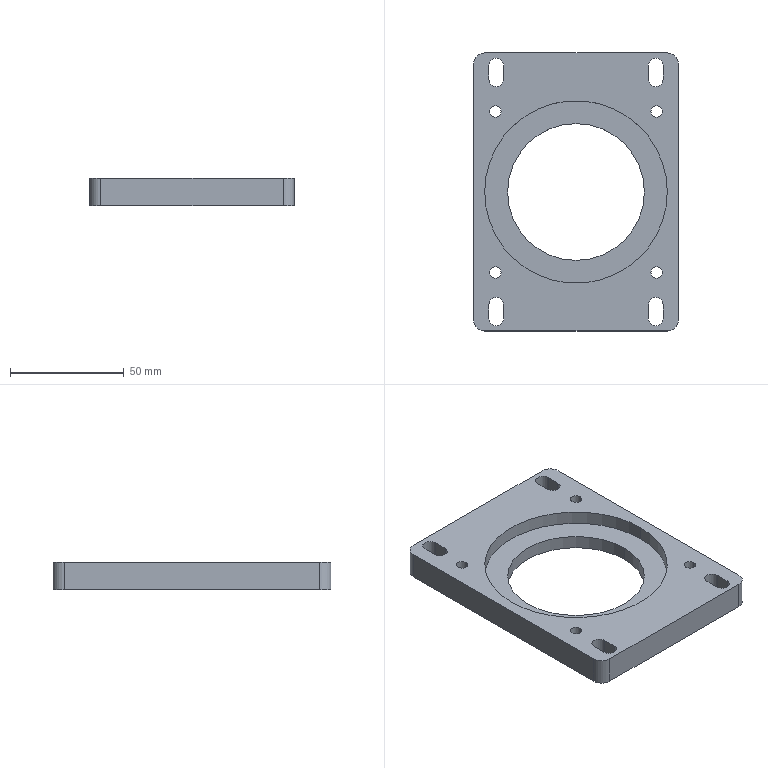Part | SolidWorks | features ICE 3, Extrusion 1, Fillet 1, HoleWzd 1 | 1 solid | 39 faces | box 90 x 122 x 12 mm | volume 79896 mm3 | cylinder 24 | plane 15 | commonest cylinder face diameters 5 x8 6.5 x8 10 x4 60 x2 80.1 x2
STEP:
#1=CARTESIAN_POINT('',(32.855,35.355,0.));
#2=VERTEX_POINT('',#1);
#3=CARTESIAN_POINT('',(37.855,35.355,0.));
#4=VERTEX_POINT('',#3);
#5=CARTESIAN_POINT('',(35.355,35.355,0.));
#6=DIRECTION('',(0.,0.,1.));
#7=DIRECTION('',(1.,0.,0.));
#8=AXIS2_PLACEMENT_3D('',#5,#6,#7);
#9=CIRCLE('',#8,2.5);
#10=EDGE_CURVE('',#2,#4,#9,.T.);
#11=ORIENTED_EDGE('',*,*,#10,.F.);
#12=CARTESIAN_POINT('',(32.855,35.355,12.));
#13=VERTEX_POINT('',#12);
#14=CARTESIAN_POINT('',(32.855,35.355,12.));
#15=DIRECTION('',(0.,0.,1.));
#16=VECTOR('',#15,1000.);
#17=LINE('',#14,#16);
#18=EDGE_CURVE('',#2,#13,#17,.T.);
#19=ORIENTED_EDGE('',*,*,#18,.T.);
#20=CARTESIAN_POINT('',(37.855,35.355,12.));
#21=VERTEX_POINT('',#20);
#22=CARTESIAN_POINT('',(35.355,35.355,12.));
#23=DIRECTION('',(0.,0.,1.));
#24=DIRECTION('',(1.,0.,0.));
#25=AXIS2_PLACEMENT_3D('',#22,#23,#24);
#26=CIRCLE('',#25,2.5);
#27=EDGE_CURVE('',#13,#21,#26,.T.);
#28=ORIENTED_EDGE('',*,*,#27,.T.);
#29=CARTESIAN_POINT('',(37.855,35.355,12.));
#30=DIRECTION('',(0.,0.,1.));
#31=VECTOR('',#30,1000.);
#32=LINE('',#29,#31);
#33=EDGE_CURVE('',#4,#21,#32,.T.);
#34=ORIENTED_EDGE('',*,*,#33,.F.);
#35=EDGE_LOOP('',(#11,#19,#28,#34));
#36=FACE_OUTER_BOUND('',#35,.T.);
#37=CARTESIAN_POINT('',(35.355,35.355,12.));
#38=DIRECTION('',(0.,0.,1.));
#39=DIRECTION('',(1.,0.,0.));
#40=AXIS2_PLACEMENT_3D('',#37,#38,#39);
#41=CYLINDRICAL_SURFACE('',#40,2.5);
#42=ADVANCED_FACE('',(#36),#41,.F.);
#43=CARTESIAN_POINT('',(-37.855,35.355,0.));
#44=VERTEX_POINT('',#43);
#45=CARTESIAN_POINT('',(-32.855,35.355,0.));
#46=VERTEX_POINT('',#45);
#47=CARTESIAN_POINT('',(-35.355,35.355,0.));
#48=DIRECTION('',(0.,0.,1.));
#49=DIRECTION('',(1.,0.,0.));
#50=AXIS2_PLACEMENT_3D('',#47,#48,#49);
#51=CIRCLE('',#50,2.5);
#52=EDGE_CURVE('',#44,#46,#51,.T.);
#53=ORIENTED_EDGE('',*,*,#52,.F.);
#54=CARTESIAN_POINT('',(-37.855,35.355,12.));
#55=VERTEX_POINT('',#54);
#56=CARTESIAN_POINT('',(-37.855,35.355,12.));
#57=DIRECTION('',(0.,0.,1.));
#58=VECTOR('',#57,1000.);
#59=LINE('',#56,#58);
#60=EDGE_CURVE('',#44,#55,#59,.T.);
#61=ORIENTED_EDGE('',*,*,#60,.T.);
#62=CARTESIAN_POINT('',(-32.855,35.355,12.));
#63=VERTEX_POINT('',#62);
#64=CARTESIAN_POINT('',(-35.355,35.355,12.));
#65=DIRECTION('',(0.,0.,1.));
#66=DIRECTION('',(1.,0.,0.));
#67=AXIS2_PLACEMENT_3D('',#64,#65,#66);
#68=CIRCLE('',#67,2.5);
#69=EDGE_CURVE('',#55,#63,#68,.T.);
#70=ORIENTED_EDGE('',*,*,#69,.T.);
#71=CARTESIAN_POINT('',(-32.855,35.355,12.));
#72=DIRECTION('',(0.,0.,1.));
#73=VECTOR('',#72,1000.);
#74=LINE('',#71,#73);
#75=EDGE_CURVE('',#46,#63,#74,.T.);
#76=ORIENTED_EDGE('',*,*,#75,.F.);
#77=EDGE_LOOP('',(#53,#61,#70,#76));
#78=FACE_OUTER_BOUND('',#77,.T.);
#79=CARTESIAN_POINT('',(-35.355,35.355,12.));
#80=DIRECTION('',(0.,0.,1.));
#81=DIRECTION('',(1.,0.,0.));
#82=AXIS2_PLACEMENT_3D('',#79,#80,#81);
#83=CYLINDRICAL_SURFACE('',#82,2.5);
#84=ADVANCED_FACE('',(#78),#83,.F.);
#85=CARTESIAN_POINT('',(-37.855,-35.355,0.));
#86=VERTEX_POINT('',#85);
#87=CARTESIAN_POINT('',(-32.855,-35.355,0.));
#88=VERTEX_POINT('',#87);
#89=CARTESIAN_POINT('',(-35.355,-35.355,0.));
#90=DIRECTION('',(0.,0.,1.));
#91=DIRECTION('',(1.,0.,0.));
#92=AXIS2_PLACEMENT_3D('',#89,#90,#91);
#93=CIRCLE('',#92,2.5);
#94=EDGE_CURVE('',#86,#88,#93,.T.);
#95=ORIENTED_EDGE('',*,*,#94,.F.);
#96=CARTESIAN_POINT('',(-37.855,-35.355,12.));
#97=VERTEX_POINT('',#96);
#98=CARTESIAN_POINT('',(-37.855,-35.355,12.));
#99=DIRECTION('',(0.,0.,1.));
#100=VECTOR('',#99,1000.);
#101=LINE('',#98,#100);
#102=EDGE_CURVE('',#86,#97,#101,.T.);
#103=ORIENTED_EDGE('',*,*,#102,.T.);
#104=CARTESIAN_POINT('',(-32.855,-35.355,12.));
#105=VERTEX_POINT('',#104);
#106=CARTESIAN_POINT('',(-35.355,-35.355,12.));
#107=DIRECTION('',(0.,0.,1.));
#108=DIRECTION('',(1.,0.,0.));
#109=AXIS2_PLACEMENT_3D('',#106,#107,#108);
#110=CIRCLE('',#109,2.5);
#111=EDGE_CURVE('',#97,#105,#110,.T.);
#112=ORIENTED_EDGE('',*,*,#111,.T.);
#113=CARTESIAN_POINT('',(-32.855,-35.355,12.));
#114=DIRECTION('',(0.,0.,1.));
#115=VECTOR('',#114,1000.);
#116=LINE('',#113,#115);
#117=EDGE_CURVE('',#88,#105,#116,.T.);
#118=ORIENTED_EDGE('',*,*,#117,.F.);
#119=EDGE_LOOP('',(#95,#103,#112,#118));
#120=FACE_OUTER_BOUND('',#119,.T.);
#121=CARTESIAN_POINT('',(-35.355,-35.355,12.));
#122=DIRECTION('',(0.,0.,1.));
#123=DIRECTION('',(1.,0.,0.));
#124=AXIS2_PLACEMENT_3D('',#121,#122,#123);
#125=CYLINDRICAL_SURFACE('',#124,2.5);
#126=ADVANCED_FACE('',(#120),#125,.F.);
#127=CARTESIAN_POINT('',(32.855,-35.355,0.));
#128=VERTEX_POINT('',#127);
#129=CARTESIAN_POINT('',(37.855,-35.355,0.));
#130=VERTEX_POINT('',#129);
#131=CARTESIAN_POINT('',(35.355,-35.355,0.));
#132=DIRECTION('',(0.,0.,1.));
#133=DIRECTION('',(1.,0.,0.));
#134=AXIS2_PLACEMENT_3D('',#131,#132,#133);
#135=CIRCLE('',#134,2.5);
#136=EDGE_CURVE('',#128,#130,#135,.T.);
#137=ORIENTED_EDGE('',*,*,#136,.F.);
#138=CARTESIAN_POINT('',(32.855,-35.355,12.));
#139=VERTEX_POINT('',#138);
#140=CARTESIAN_POINT('',(32.855,-35.355,12.));
#141=DIRECTION('',(0.,0.,1.));
#142=VECTOR('',#141,1000.);
#143=LINE('',#140,#142);
#144=EDGE_CURVE('',#128,#139,#143,.T.);
#145=ORIENTED_EDGE('',*,*,#144,.T.);
#146=CARTESIAN_POINT('',(37.855,-35.355,12.));
#147=VERTEX_POINT('',#146);
#148=CARTESIAN_POINT('',(35.355,-35.355,12.));
#149=DIRECTION('',(0.,0.,1.));
#150=DIRECTION('',(1.,0.,0.));
#151=AXIS2_PLACEMENT_3D('',#148,#149,#150);
#152=CIRCLE('',#151,2.5);
#153=EDGE_CURVE('',#139,#147,#152,.T.);
#154=ORIENTED_EDGE('',*,*,#153,.T.);
#155=CARTESIAN_POINT('',(37.855,-35.355,12.));
#156=DIRECTION('',(0.,0.,1.));
#157=VECTOR('',#156,1000.);
#158=LINE('',#155,#157);
#159=EDGE_CURVE('',#130,#147,#158,.T.);
#160=ORIENTED_EDGE('',*,*,#159,.F.);
#161=EDGE_LOOP('',(#137,#145,#154,#160));
#162=FACE_OUTER_BOUND('',#161,.T.);
#163=CARTESIAN_POINT('',(35.355,-35.355,12.));
#164=DIRECTION('',(0.,0.,1.));
#165=DIRECTION('',(1.,0.,0.));
#166=AXIS2_PLACEMENT_3D('',#163,#164,#165);
#167=CYLINDRICAL_SURFACE('',#166,2.5);
#168=ADVANCED_FACE('',(#162),#167,.F.);
#169=CARTESIAN_POINT('',(-40.05,0.,6.));
#170=VERTEX_POINT('',#169);
#171=CARTESIAN_POINT('',(40.05,0.,6.));
#172=VERTEX_POINT('',#171);
#173=CARTESIAN_POINT('',(0.,0.,6.));
#174=DIRECTION('',(0.,0.,1.));
#175=DIRECTION('',(1.,0.,0.));
#176=AXIS2_PLACEMENT_3D('',#173,#174,#175);
#177=CIRCLE('',#176,40.05);
#178=EDGE_CURVE('',#170,#172,#177,.T.);
#179=ORIENTED_EDGE('',*,*,#178,.F.);
#180=CARTESIAN_POINT('',(-40.05,0.,12.));
#181=VERTEX_POINT('',#180);
#182=CARTESIAN_POINT('',(-40.05,0.,6.));
#183=DIRECTION('',(0.,0.,1.));
#184=VECTOR('',#183,1000.);
#185=LINE('',#182,#184);
#186=EDGE_CURVE('',#170,#181,#185,.T.);
#187=ORIENTED_EDGE('',*,*,#186,.T.);
#188=CARTESIAN_POINT('',(40.05,0.,12.));
#189=VERTEX_POINT('',#188);
#190=CARTESIAN_POINT('',(0.,0.,12.));
#191=DIRECTION('',(0.,0.,1.));
#192=DIRECTION('',(1.,0.,0.));
#193=AXIS2_PLACEMENT_3D('',#190,#191,#192);
#194=CIRCLE('',#193,40.05);
#195=EDGE_CURVE('',#181,#189,#194,.T.);
#196=ORIENTED_EDGE('',*,*,#195,.T.);
#197=CARTESIAN_POINT('',(40.05,0.,6.));
#198=DIRECTION('',(0.,0.,1.));
#199=VECTOR('',#198,1000.);
#200=LINE('',#197,#199);
#201=EDGE_CURVE('',#172,#189,#200,.T.);
#202=ORIENTED_EDGE('',*,*,#201,.F.);
#203=EDGE_LOOP('',(#179,#187,#196,#202));
#204=FACE_OUTER_BOUND('',#203,.T.);
#205=CARTESIAN_POINT('',(0.,0.,6.));
#206=DIRECTION('',(0.,0.,1.));
#207=DIRECTION('',(1.,0.,0.));
#208=AXIS2_PLACEMENT_3D('',#205,#206,#207);
#209=CYLINDRICAL_SURFACE('',#208,40.05);
#210=ADVANCED_FACE('',(#204),#209,.F.);
#211=CARTESIAN_POINT('',(-30.,0.,0.));
#212=VERTEX_POINT('',#211);
#213=CARTESIAN_POINT('',(30.,0.,0.));
#214=VERTEX_POINT('',#213);
#215=CARTESIAN_POINT('',(0.,0.,0.));
#216=DIRECTION('',(0.,0.,1.));
#217=DIRECTION('',(1.,0.,0.));
#218=AXIS2_PLACEMENT_3D('',#215,#216,#217);
#219=CIRCLE('',#218,30.);
#220=EDGE_CURVE('',#212,#214,#219,.T.);
#221=ORIENTED_EDGE('',*,*,#220,.F.);
#222=CARTESIAN_POINT('',(-30.,0.,6.));
#223=VERTEX_POINT('',#222);
#224=CARTESIAN_POINT('',(-30.,0.,0.));
#225=DIRECTION('',(0.,0.,1.));
#226=VECTOR('',#225,1000.);
#227=LINE('',#224,#226);
#228=EDGE_CURVE('',#212,#223,#227,.T.);
#229=ORIENTED_EDGE('',*,*,#228,.T.);
#230=CARTESIAN_POINT('',(30.,0.,6.));
#231=VERTEX_POINT('',#230);
#232=CARTESIAN_POINT('',(0.,0.,6.));
#233=DIRECTION('',(0.,0.,-1.));
#234=DIRECTION('',(1.,0.,0.));
#235=AXIS2_PLACEMENT_3D('',#232,#233,#234);
#236=CIRCLE('',#235,30.);
#237=EDGE_CURVE('',#231,#223,#236,.T.);
#238=ORIENTED_EDGE('',*,*,#237,.F.);
#239=CARTESIAN_POINT('',(30.,0.,0.));
#240=DIRECTION('',(0.,0.,1.));
#241=VECTOR('',#240,1000.);
#242=LINE('',#239,#241);
#243=EDGE_CURVE('',#214,#231,#242,.T.);
#244=ORIENTED_EDGE('',*,*,#243,.F.);
#245=EDGE_LOOP('',(#221,#229,#238,#244));
#246=FACE_OUTER_BOUND('',#245,.T.);
#247=CARTESIAN_POINT('',(0.,0.,0.));
#248=DIRECTION('',(0.,0.,1.));
#249=DIRECTION('',(1.,0.,0.));
#250=AXIS2_PLACEMENT_3D('',#247,#248,#249);
#251=CYLINDRICAL_SURFACE('',#250,30.);
#252=ADVANCED_FACE('',(#246),#251,.F.);
#253=CARTESIAN_POINT('',(38.25,-55.5,12.));
#254=VERTEX_POINT('',#253);
#255=CARTESIAN_POINT('',(38.25,-49.5,12.));
#256=VERTEX_POINT('',#255);
#257=CARTESIAN_POINT('',(38.25,0.,12.));
#258=DIRECTION('',(0.,1.,0.));
#259=VECTOR('',#258,1000.);
#260=LINE('',#257,#259);
#261=EDGE_CURVE('',#254,#256,#260,.T.);
#262=ORIENTED_EDGE('',*,*,#261,.F.);
#263=CARTESIAN_POINT('',(31.75,-55.5,12.));
#264=VERTEX_POINT('',#263);
#265=CARTESIAN_POINT('',(35.,-55.5,12.));
#266=DIRECTION('',(0.,0.,1.));
#267=DIRECTION('',(1.,0.,0.));
#268=AXIS2_PLACEMENT_3D('',#265,#266,#267);
#269=CIRCLE('',#268,3.25);
#270=EDGE_CURVE('',#264,#254,#269,.T.);
#271=ORIENTED_EDGE('',*,*,#270,.F.);
#272=CARTESIAN_POINT('',(31.75,-49.5,12.));
#273=VERTEX_POINT('',#272);
#274=CARTESIAN_POINT('',(31.75,0.,12.));
#275=DIRECTION('',(0.,1.,0.));
#276=VECTOR('',#275,1000.);
#277=LINE('',#274,#276);
#278=EDGE_CURVE('',#264,#273,#277,.T.);
#279=ORIENTED_EDGE('',*,*,#278,.T.);
#280=CARTESIAN_POINT('',(35.,-49.5,12.));
#281=DIRECTION('',(0.,0.,1.));
#282=DIRECTION('',(1.,0.,0.));
#283=AXIS2_PLACEMENT_3D('',#280,#281,#282);
#284=CIRCLE('',#283,3.25);
#285=EDGE_CURVE('',#256,#273,#284,.T.);
#286=ORIENTED_EDGE('',*,*,#285,.F.);
#287=EDGE_LOOP('',(#262,#271,#279,#286));
#288=FACE_BOUND('',#287,.T.);
#289=CARTESIAN_POINT('',(-38.25,55.5,12.));
#290=VERTEX_POINT('',#289);
#291=CARTESIAN_POINT('',(-38.25,49.5,12.));
#292=VERTEX_POINT('',#291);
#293=CARTESIAN_POINT('',(-38.25,0.,12.));
#294=DIRECTION('',(0.,-1.,0.));
#295=VECTOR('',#294,1000.);
#296=LINE('',#293,#295);
#297=EDGE_CURVE('',#290,#292,#296,.T.);
#298=ORIENTED_EDGE('',*,*,#297,.F.);
#299=CARTESIAN_POINT('',(-31.75,55.5,12.));
#300=VERTEX_POINT('',#299);
#301=CARTESIAN_POINT('',(-35.,55.5,12.));
#302=DIRECTION('',(0.,0.,1.));
#303=DIRECTION('',(1.,0.,0.));
#304=AXIS2_PLACEMENT_3D('',#301,#302,#303);
#305=CIRCLE('',#304,3.25);
#306=EDGE_CURVE('',#300,#290,#305,.T.);
#307=ORIENTED_EDGE('',*,*,#306,.F.);
#308=CARTESIAN_POINT('',(-31.75,49.5,12.));
#309=VERTEX_POINT('',#308);
#310=CARTESIAN_POINT('',(-31.75,0.,12.));
#311=DIRECTION('',(0.,-1.,0.));
#312=VECTOR('',#311,1000.);
#313=LINE('',#310,#312);
#314=EDGE_CURVE('',#300,#309,#313,.T.);
#315=ORIENTED_EDGE('',*,*,#314,.T.);
#316=CARTESIAN_POINT('',(-35.,49.5,12.));
#317=DIRECTION('',(0.,0.,1.));
#318=DIRECTION('',(1.,0.,0.));
#319=AXIS2_PLACEMENT_3D('',#316,#317,#318);
#320=CIRCLE('',#319,3.25);
#321=EDGE_CURVE('',#292,#309,#320,.T.);
#322=ORIENTED_EDGE('',*,*,#321,.F.);
#323=EDGE_LOOP('',(#298,#307,#315,#322));
#324=FACE_BOUND('',#323,.T.);
#325=CARTESIAN_POINT('',(35.355,35.355,12.));
#326=DIRECTION('',(0.,0.,1.));
#327=DIRECTION('',(1.,0.,0.));
#328=AXIS2_PLACEMENT_3D('',#325,#326,#327);
#329=CIRCLE('',#328,2.5);
#330=EDGE_CURVE('',#21,#13,#329,.T.);
#331=ORIENTED_EDGE('',*,*,#330,.F.);
#332=ORIENTED_EDGE('',*,*,#27,.F.);
#333=EDGE_LOOP('',(#331,#332));
#334=FACE_BOUND('',#333,.T.);
#335=CARTESIAN_POINT('',(-35.355,35.355,12.));
#336=DIRECTION('',(0.,0.,1.));
#337=DIRECTION('',(1.,0.,0.));
#338=AXIS2_PLACEMENT_3D('',#335,#336,#337);
#339=CIRCLE('',#338,2.5);
#340=EDGE_CURVE('',#63,#55,#339,.T.);
#341=ORIENTED_EDGE('',*,*,#340,.F.);
#342=ORIENTED_EDGE('',*,*,#69,.F.);
#343=EDGE_LOOP('',(#341,#342));
#344=FACE_BOUND('',#343,.T.);
#345=CARTESIAN_POINT('',(-35.355,-35.355,12.));
#346=DIRECTION('',(0.,0.,1.));
#347=DIRECTION('',(1.,0.,0.));
#348=AXIS2_PLACEMENT_3D('',#345,#346,#347);
#349=CIRCLE('',#348,2.5);
#350=EDGE_CURVE('',#105,#97,#349,.T.);
#351=ORIENTED_EDGE('',*,*,#350,.F.);
#352=ORIENTED_EDGE('',*,*,#111,.F.);
#353=EDGE_LOOP('',(#351,#352));
#354=FACE_BOUND('',#353,.T.);
#355=CARTESIAN_POINT('',(35.355,-35.355,12.));
#356=DIRECTION('',(0.,0.,1.));
#357=DIRECTION('',(1.,0.,0.));
#358=AXIS2_PLACEMENT_3D('',#355,#356,#357);
#359=CIRCLE('',#358,2.5);
#360=EDGE_CURVE('',#147,#139,#359,.T.);
#361=ORIENTED_EDGE('',*,*,#360,.F.);
#362=ORIENTED_EDGE('',*,*,#153,.F.);
#363=EDGE_LOOP('',(#361,#362));
#364=FACE_BOUND('',#363,.T.);
#365=CARTESIAN_POINT('',(0.,0.,12.));
#366=DIRECTION('',(0.,0.,1.));
#367=DIRECTION('',(1.,0.,0.));
#368=AXIS2_PLACEMENT_3D('',#365,#366,#367);
#369=CIRCLE('',#368,40.05);
#370=EDGE_CURVE('',#189,#181,#369,.T.);
#371=ORIENTED_EDGE('',*,*,#370,.F.);
#372=ORIENTED_EDGE('',*,*,#195,.F.);
#373=EDGE_LOOP('',(#371,#372));
#374=FACE_BOUND('',#373,.T.);
#375=CARTESIAN_POINT('',(40.,61.,12.));
#376=VERTEX_POINT('',#375);
#377=CARTESIAN_POINT('',(-40.,61.,12.));
#378=VERTEX_POINT('',#377);
#379=CARTESIAN_POINT('',(-45.,61.,12.));
#380=DIRECTION('',(-1.,0.,0.));
#381=VECTOR('',#380,1000.);
#382=LINE('',#379,#381);
#383=EDGE_CURVE('',#376,#378,#382,.T.);
#384=ORIENTED_EDGE('',*,*,#383,.T.);
#385=CARTESIAN_POINT('',(-45.,56.,12.));
#386=VERTEX_POINT('',#385);
#387=CARTESIAN_POINT('',(-40.,56.,12.));
#388=DIRECTION('',(0.,0.,1.));
#389=DIRECTION('',(1.,0.,0.));
#390=AXIS2_PLACEMENT_3D('',#387,#388,#389);
#391=CIRCLE('',#390,5.);
#392=EDGE_CURVE('',#378,#386,#391,.T.);
#393=ORIENTED_EDGE('',*,*,#392,.T.);
#394=CARTESIAN_POINT('',(-45.,-56.,12.));
#395=VERTEX_POINT('',#394);
#396=CARTESIAN_POINT('',(-45.,61.,12.));
#397=DIRECTION('',(0.,-1.,0.));
#398=VECTOR('',#397,1000.);
#399=LINE('',#396,#398);
#400=EDGE_CURVE('',#386,#395,#399,.T.);
#401=ORIENTED_EDGE('',*,*,#400,.T.);
#402=CARTESIAN_POINT('',(-40.,-61.,12.));
#403=VERTEX_POINT('',#402);
#404=CARTESIAN_POINT('',(-40.,-56.,12.));
#405=DIRECTION('',(0.,0.,1.));
#406=DIRECTION('',(1.,0.,0.));
#407=AXIS2_PLACEMENT_3D('',#404,#405,#406);
#408=CIRCLE('',#407,5.);
#409=EDGE_CURVE('',#395,#403,#408,.T.);
#410=ORIENTED_EDGE('',*,*,#409,.T.);
#411=CARTESIAN_POINT('',(40.,-61.,12.));
#412=VERTEX_POINT('',#411);
#413=CARTESIAN_POINT('',(-45.,-61.,12.));
#414=DIRECTION('',(1.,0.,0.));
#415=VECTOR('',#414,1000.);
#416=LINE('',#413,#415);
#417=EDGE_CURVE('',#403,#412,#416,.T.);
#418=ORIENTED_EDGE('',*,*,#417,.T.);
#419=CARTESIAN_POINT('',(45.,-56.,12.));
#420=VERTEX_POINT('',#419);
#421=CARTESIAN_POINT('',(40.,-56.,12.));
#422=DIRECTION('',(0.,0.,1.));
#423=DIRECTION('',(1.,0.,0.));
#424=AXIS2_PLACEMENT_3D('',#421,#422,#423);
#425=CIRCLE('',#424,5.);
#426=EDGE_CURVE('',#412,#420,#425,.T.);
#427=ORIENTED_EDGE('',*,*,#426,.T.);
#428=CARTESIAN_POINT('',(45.,56.,12.));
#429=VERTEX_POINT('',#428);
#430=CARTESIAN_POINT('',(45.,61.,12.));
#431=DIRECTION('',(0.,1.,0.));
#432=VECTOR('',#431,1000.);
#433=LINE('',#430,#432);
#434=EDGE_CURVE('',#420,#429,#433,.T.);
#435=ORIENTED_EDGE('',*,*,#434,.T.);
#436=CARTESIAN_POINT('',(40.,56.,12.));
#437=DIRECTION('',(0.,0.,1.));
#438=DIRECTION('',(1.,0.,0.));
#439=AXIS2_PLACEMENT_3D('',#436,#437,#438);
#440=CIRCLE('',#439,5.);
#441=EDGE_CURVE('',#429,#376,#440,.T.);
#442=ORIENTED_EDGE('',*,*,#441,.T.);
#443=EDGE_LOOP('',(#384,#393,#401,#410,#418,#427,#435,#442));
#444=FACE_OUTER_BOUND('',#443,.T.);
#445=CARTESIAN_POINT('',(38.25,55.5,12.));
#446=VERTEX_POINT('',#445);
#447=CARTESIAN_POINT('',(38.25,49.5,12.));
#448=VERTEX_POINT('',#447);
#449=CARTESIAN_POINT('',(38.25,0.,12.));
#450=DIRECTION('',(0.,-1.,0.));
#451=VECTOR('',#450,1000.);
#452=LINE('',#449,#451);
#453=EDGE_CURVE('',#446,#448,#452,.T.);
#454=ORIENTED_EDGE('',*,*,#453,.T.);
#455=CARTESIAN_POINT('',(31.75,49.5,12.));
#456=VERTEX_POINT('',#455);
#457=CARTESIAN_POINT('',(35.,49.5,12.));
#458=DIRECTION('',(0.,0.,-1.));
#459=DIRECTION('',(1.,0.,0.));
#460=AXIS2_PLACEMENT_3D('',#457,#458,#459);
#461=CIRCLE('',#460,3.25);
#462=EDGE_CURVE('',#448,#456,#461,.T.);
#463=ORIENTED_EDGE('',*,*,#462,.T.);
#464=CARTESIAN_POINT('',(31.75,55.5,12.));
#465=VERTEX_POINT('',#464);
#466=CARTESIAN_POINT('',(31.75,0.,12.));
#467=DIRECTION('',(0.,-1.,0.));
#468=VECTOR('',#467,1000.);
#469=LINE('',#466,#468);
#470=EDGE_CURVE('',#465,#456,#469,.T.);
#471=ORIENTED_EDGE('',*,*,#470,.F.);
#472=CARTESIAN_POINT('',(35.,55.5,12.));
#473=DIRECTION('',(0.,0.,-1.));
#474=DIRECTION('',(1.,0.,0.));
#475=AXIS2_PLACEMENT_3D('',#472,#473,#474);
#476=CIRCLE('',#475,3.25);
#477=EDGE_CURVE('',#465,#446,#476,.T.);
#478=ORIENTED_EDGE('',*,*,#477,.T.);
#479=EDGE_LOOP('',(#454,#463,#471,#478));
#480=FACE_BOUND('',#479,.T.);
#481=CARTESIAN_POINT('',(-38.25,-55.5,12.));
#482=VERTEX_POINT('',#481);
#483=CARTESIAN_POINT('',(-38.25,-49.5,12.));
#484=VERTEX_POINT('',#483);
#485=CARTESIAN_POINT('',(-38.25,0.,12.));
#486=DIRECTION('',(0.,1.,0.));
#487=VECTOR('',#486,1000.);
#488=LINE('',#485,#487);
#489=EDGE_CURVE('',#482,#484,#488,.T.);
#490=ORIENTED_EDGE('',*,*,#489,.T.);
#491=CARTESIAN_POINT('',(-31.75,-49.5,12.));
#492=VERTEX_POINT('',#491);
#493=CARTESIAN_POINT('',(-35.,-49.5,12.));
#494=DIRECTION('',(0.,0.,-1.));
#495=DIRECTION('',(1.,0.,0.));
#496=AXIS2_PLACEMENT_3D('',#493,#494,#495);
#497=CIRCLE('',#496,3.25);
#498=EDGE_CURVE('',#484,#492,#497,.T.);
#499=ORIENTED_EDGE('',*,*,#498,.T.);
#500=CARTESIAN_POINT('',(-31.75,-55.5,12.));
#501=VERTEX_POINT('',#500);
#502=CARTESIAN_POINT('',(-31.75,0.,12.));
#503=DIRECTION('',(0.,1.,0.));
#504=VECTOR('',#503,1000.);
#505=LINE('',#502,#504);
#506=EDGE_CURVE('',#501,#492,#505,.T.);
#507=ORIENTED_EDGE('',*,*,#506,.F.);
#508=CARTESIAN_POINT('',(-35.,-55.5,12.));
#509=DIRECTION('',(0.,0.,-1.));
#510=DIRECTION('',(1.,0.,0.));
#511=AXIS2_PLACEMENT_3D('',#508,#509,#510);
#512=CIRCLE('',#511,3.25);
#513=EDGE_CURVE('',#501,#482,#512,.T.);
#514=ORIENTED_EDGE('',*,*,#513,.T.);
#515=EDGE_LOOP('',(#490,#499,#507,#514));
#516=FACE_BOUND('',#515,.T.);
#517=CARTESIAN_POINT('',(0.,0.,12.));
#518=DIRECTION('',(0.,0.,1.));
#519=DIRECTION('',(1.,0.,0.));
#520=AXIS2_PLACEMENT_3D('',#517,#518,#519);
#521=PLANE('',#520);
#522=ADVANCED_FACE('',(#288,#324,#334,#344,#354,#364,#374,#444,#480,#516),#521,.T.);
#523=CARTESIAN_POINT('',(38.25,49.5,0.));
#524=VERTEX_POINT('',#523);
#525=CARTESIAN_POINT('',(31.75,49.5,0.));
#526=VERTEX_POINT('',#525);
#527=CARTESIAN_POINT('',(35.,49.5,0.));
#528=DIRECTION('',(0.,0.,-1.));
#529=DIRECTION('',(1.,0.,0.));
#530=AXIS2_PLACEMENT_3D('',#527,#528,#529);
#531=CIRCLE('',#530,3.25);
#532=EDGE_CURVE('',#524,#526,#531,.T.);
#533=ORIENTED_EDGE('',*,*,#532,.F.);
#534=CARTESIAN_POINT('',(38.25,55.5,0.));
#535=VERTEX_POINT('',#534);
#536=CARTESIAN_POINT('',(38.25,0.,0.));
#537=DIRECTION('',(0.,-1.,0.));
#538=VECTOR('',#537,1000.);
#539=LINE('',#536,#538);
#540=EDGE_CURVE('',#535,#524,#539,.T.);
#541=ORIENTED_EDGE('',*,*,#540,.F.);
#542=CARTESIAN_POINT('',(31.75,55.5,0.));
#543=VERTEX_POINT('',#542);
#544=CARTESIAN_POINT('',(35.,55.5,0.));
#545=DIRECTION('',(0.,0.,-1.));
#546=DIRECTION('',(1.,0.,0.));
#547=AXIS2_PLACEMENT_3D('',#544,#545,#546);
#548=CIRCLE('',#547,3.25);
#549=EDGE_CURVE('',#543,#535,#548,.T.);
#550=ORIENTED_EDGE('',*,*,#549,.F.);
#551=CARTESIAN_POINT('',(31.75,0.,0.));
#552=DIRECTION('',(0.,-1.,0.));
#553=VECTOR('',#552,1000.);
#554=LINE('',#551,#553);
#555=EDGE_CURVE('',#543,#526,#554,.T.);
#556=ORIENTED_EDGE('',*,*,#555,.T.);
#557=EDGE_LOOP('',(#533,#541,#550,#556));
#558=FACE_BOUND('',#557,.T.);
#559=CARTESIAN_POINT('',(-31.75,55.5,0.));
#560=VERTEX_POINT('',#559);
#561=CARTESIAN_POINT('',(-38.25,55.5,0.));
#562=VERTEX_POINT('',#561);
#563=CARTESIAN_POINT('',(-35.,55.5,0.));
#564=DIRECTION('',(0.,0.,1.));
#565=DIRECTION('',(1.,0.,0.));
#566=AXIS2_PLACEMENT_3D('',#563,#564,#565);
#567=CIRCLE('',#566,3.25);
#568=EDGE_CURVE('',#560,#562,#567,.T.);
#569=ORIENTED_EDGE('',*,*,#568,.T.);
#570=CARTESIAN_POINT('',(-38.25,49.5,0.));
#571=VERTEX_POINT('',#570);
#572=CARTESIAN_POINT('',(-38.25,0.,0.));
#573=DIRECTION('',(0.,-1.,0.));
#574=VECTOR('',#573,1000.);
#575=LINE('',#572,#574);
#576=EDGE_CURVE('',#562,#571,#575,.T.);
#577=ORIENTED_EDGE('',*,*,#576,.T.);
#578=CARTESIAN_POINT('',(-31.75,49.5,0.));
#579=VERTEX_POINT('',#578);
#580=CARTESIAN_POINT('',(-35.,49.5,0.));
#581=DIRECTION('',(0.,0.,1.));
#582=DIRECTION('',(1.,0.,0.));
#583=AXIS2_PLACEMENT_3D('',#580,#581,#582);
#584=CIRCLE('',#583,3.25);
#585=EDGE_CURVE('',#571,#579,#584,.T.);
#586=ORIENTED_EDGE('',*,*,#585,.T.);
#587=CARTESIAN_POINT('',(-31.75,0.,0.));
#588=DIRECTION('',(0.,-1.,0.));
#589=VECTOR('',#588,1000.);
#590=LINE('',#587,#589);
#591=EDGE_CURVE('',#560,#579,#590,.T.);
#592=ORIENTED_EDGE('',*,*,#591,.F.);
#593=EDGE_LOOP('',(#569,#577,#586,#592));
#594=FACE_BOUND('',#593,.T.);
#595=CARTESIAN_POINT('',(35.355,35.355,0.));
#596=DIRECTION('',(0.,0.,1.));
#597=DIRECTION('',(1.,0.,0.));
#598=AXIS2_PLACEMENT_3D('',#595,#596,#597);
#599=CIRCLE('',#598,2.5);
#600=EDGE_CURVE('',#4,#2,#599,.T.);
#601=ORIENTED_EDGE('',*,*,#600,.T.);
#602=ORIENTED_EDGE('',*,*,#10,.T.);
#603=EDGE_LOOP('',(#601,#602));
#604=FACE_BOUND('',#603,.T.);
#605=CARTESIAN_POINT('',(-35.355,35.355,0.));
#606=DIRECTION('',(0.,0.,1.));
#607=DIRECTION('',(1.,0.,0.));
#608=AXIS2_PLACEMENT_3D('',#605,#606,#607);
#609=CIRCLE('',#608,2.5);
#610=EDGE_CURVE('',#46,#44,#609,.T.);
#611=ORIENTED_EDGE('',*,*,#610,.T.);
#612=ORIENTED_EDGE('',*,*,#52,.T.);
#613=EDGE_LOOP('',(#611,#612));
#614=FACE_BOUND('',#613,.T.);
#615=CARTESIAN_POINT('',(-35.355,-35.355,0.));
#616=DIRECTION('',(0.,0.,1.));
#617=DIRECTION('',(1.,0.,0.));
#618=AXIS2_PLACEMENT_3D('',#615,#616,#617);
#619=CIRCLE('',#618,2.5);
#620=EDGE_CURVE('',#88,#86,#619,.T.);
#621=ORIENTED_EDGE('',*,*,#620,.T.);
#622=ORIENTED_EDGE('',*,*,#94,.T.);
#623=EDGE_LOOP('',(#621,#622));
#624=FACE_BOUND('',#623,.T.);
#625=CARTESIAN_POINT('',(35.355,-35.355,0.));
#626=DIRECTION('',(0.,0.,1.));
#627=DIRECTION('',(1.,0.,0.));
#628=AXIS2_PLACEMENT_3D('',#625,#626,#627);
#629=CIRCLE('',#628,2.5);
#630=EDGE_CURVE('',#130,#128,#629,.T.);
#631=ORIENTED_EDGE('',*,*,#630,.T.);
#632=ORIENTED_EDGE('',*,*,#136,.T.);
#633=EDGE_LOOP('',(#631,#632));
#634=FACE_BOUND('',#633,.T.);
#635=CARTESIAN_POINT('',(0.,0.,0.));
#636=DIRECTION('',(0.,0.,1.));
#637=DIRECTION('',(1.,0.,0.));
#638=AXIS2_PLACEMENT_3D('',#635,#636,#637);
#639=CIRCLE('',#638,30.);
#640=EDGE_CURVE('',#214,#212,#639,.T.);
#641=ORIENTED_EDGE('',*,*,#640,.T.);
#642=ORIENTED_EDGE('',*,*,#220,.T.);
#643=EDGE_LOOP('',(#641,#642));
#644=FACE_BOUND('',#643,.T.);
#645=CARTESIAN_POINT('',(-45.,56.,0.));
#646=VERTEX_POINT('',#645);
#647=CARTESIAN_POINT('',(-45.,-56.,0.));
#648=VERTEX_POINT('',#647);
#649=CARTESIAN_POINT('',(-45.,61.,0.));
#650=DIRECTION('',(0.,-1.,0.));
#651=VECTOR('',#650,1000.);
#652=LINE('',#649,#651);
#653=EDGE_CURVE('',#646,#648,#652,.T.);
#654=ORIENTED_EDGE('',*,*,#653,.F.);
#655=CARTESIAN_POINT('',(-40.,61.,0.));
#656=VERTEX_POINT('',#655);
#657=CARTESIAN_POINT('',(-40.,56.,0.));
#658=DIRECTION('',(0.,0.,-1.));
#659=DIRECTION('',(1.,0.,0.));
#660=AXIS2_PLACEMENT_3D('',#657,#658,#659);
#661=CIRCLE('',#660,5.);
#662=EDGE_CURVE('',#646,#656,#661,.T.);
#663=ORIENTED_EDGE('',*,*,#662,.T.);
#664=CARTESIAN_POINT('',(40.,61.,0.));
#665=VERTEX_POINT('',#664);
#666=CARTESIAN_POINT('',(-45.,61.,0.));
#667=DIRECTION('',(-1.,0.,0.));
#668=VECTOR('',#667,1000.);
#669=LINE('',#666,#668);
#670=EDGE_CURVE('',#665,#656,#669,.T.);
#671=ORIENTED_EDGE('',*,*,#670,.F.);
#672=CARTESIAN_POINT('',(45.,56.,0.));
#673=VERTEX_POINT('',#672);
#674=CARTESIAN_POINT('',(40.,56.,0.));
#675=DIRECTION('',(0.,0.,-1.));
#676=DIRECTION('',(1.,0.,0.));
#677=AXIS2_PLACEMENT_3D('',#674,#675,#676);
#678=CIRCLE('',#677,5.);
#679=EDGE_CURVE('',#665,#673,#678,.T.);
#680=ORIENTED_EDGE('',*,*,#679,.T.);
#681=CARTESIAN_POINT('',(45.,-56.,0.));
#682=VERTEX_POINT('',#681);
#683=CARTESIAN_POINT('',(45.,61.,0.));
#684=DIRECTION('',(0.,1.,0.));
#685=VECTOR('',#684,1000.);
#686=LINE('',#683,#685);
#687=EDGE_CURVE('',#682,#673,#686,.T.);
#688=ORIENTED_EDGE('',*,*,#687,.F.);
#689=CARTESIAN_POINT('',(40.,-61.,0.));
#690=VERTEX_POINT('',#689);
#691=CARTESIAN_POINT('',(40.,-56.,0.));
#692=DIRECTION('',(0.,0.,-1.));
#693=DIRECTION('',(1.,0.,0.));
#694=AXIS2_PLACEMENT_3D('',#691,#692,#693);
#695=CIRCLE('',#694,5.);
#696=EDGE_CURVE('',#682,#690,#695,.T.);
#697=ORIENTED_EDGE('',*,*,#696,.T.);
#698=CARTESIAN_POINT('',(-40.,-61.,0.));
#699=VERTEX_POINT('',#698);
#700=CARTESIAN_POINT('',(-45.,-61.,0.));
#701=DIRECTION('',(1.,0.,0.));
#702=VECTOR('',#701,1000.);
#703=LINE('',#700,#702);
#704=EDGE_CURVE('',#699,#690,#703,.T.);
#705=ORIENTED_EDGE('',*,*,#704,.F.);
#706=CARTESIAN_POINT('',(-40.,-56.,0.));
#707=DIRECTION('',(0.,0.,-1.));
#708=DIRECTION('',(1.,0.,0.));
#709=AXIS2_PLACEMENT_3D('',#706,#707,#708);
#710=CIRCLE('',#709,5.);
#711=EDGE_CURVE('',#699,#648,#710,.T.);
#712=ORIENTED_EDGE('',*,*,#711,.T.);
#713=EDGE_LOOP('',(#654,#663,#671,#680,#688,#697,#705,#712));
#714=FACE_OUTER_BOUND('',#713,.T.);
#715=CARTESIAN_POINT('',(31.75,-55.5,0.));
#716=VERTEX_POINT('',#715);
#717=CARTESIAN_POINT('',(38.25,-55.5,0.));
#718=VERTEX_POINT('',#717);
#719=CARTESIAN_POINT('',(35.,-55.5,0.));
#720=DIRECTION('',(0.,0.,1.));
#721=DIRECTION('',(1.,0.,0.));
#722=AXIS2_PLACEMENT_3D('',#719,#720,#721);
#723=CIRCLE('',#722,3.25);
#724=EDGE_CURVE('',#716,#718,#723,.T.);
#725=ORIENTED_EDGE('',*,*,#724,.T.);
#726=CARTESIAN_POINT('',(38.25,-49.5,0.));
#727=VERTEX_POINT('',#726);
#728=CARTESIAN_POINT('',(38.25,0.,0.));
#729=DIRECTION('',(0.,1.,0.));
#730=VECTOR('',#729,1000.);
#731=LINE('',#728,#730);
#732=EDGE_CURVE('',#718,#727,#731,.T.);
#733=ORIENTED_EDGE('',*,*,#732,.T.);
#734=CARTESIAN_POINT('',(31.75,-49.5,0.));
#735=VERTEX_POINT('',#734);
#736=CARTESIAN_POINT('',(35.,-49.5,0.));
#737=DIRECTION('',(0.,0.,1.));
#738=DIRECTION('',(1.,0.,0.));
#739=AXIS2_PLACEMENT_3D('',#736,#737,#738);
#740=CIRCLE('',#739,3.25);
#741=EDGE_CURVE('',#727,#735,#740,.T.);
#742=ORIENTED_EDGE('',*,*,#741,.T.);
#743=CARTESIAN_POINT('',(31.75,0.,0.));
#744=DIRECTION('',(0.,1.,0.));
#745=VECTOR('',#744,1000.);
#746=LINE('',#743,#745);
#747=EDGE_CURVE('',#716,#735,#746,.T.);
#748=ORIENTED_EDGE('',*,*,#747,.F.);
#749=EDGE_LOOP('',(#725,#733,#742,#748));
#750=FACE_BOUND('',#749,.T.);
#751=CARTESIAN_POINT('',(-38.25,-49.5,0.));
#752=VERTEX_POINT('',#751);
#753=CARTESIAN_POINT('',(-31.75,-49.5,0.));
#754=VERTEX_POINT('',#753);
#755=CARTESIAN_POINT('',(-35.,-49.5,0.));
#756=DIRECTION('',(0.,0.,-1.));
#757=DIRECTION('',(1.,0.,0.));
#758=AXIS2_PLACEMENT_3D('',#755,#756,#757);
#759=CIRCLE('',#758,3.25);
#760=EDGE_CURVE('',#752,#754,#759,.T.);
#761=ORIENTED_EDGE('',*,*,#760,.F.);
#762=CARTESIAN_POINT('',(-38.25,-55.5,0.));
#763=VERTEX_POINT('',#762);
#764=CARTESIAN_POINT('',(-38.25,0.,0.));
#765=DIRECTION('',(0.,1.,0.));
#766=VECTOR('',#765,1000.);
#767=LINE('',#764,#766);
#768=EDGE_CURVE('',#763,#752,#767,.T.);
#769=ORIENTED_EDGE('',*,*,#768,.F.);
#770=CARTESIAN_POINT('',(-31.75,-55.5,0.));
#771=VERTEX_POINT('',#770);
#772=CARTESIAN_POINT('',(-35.,-55.5,0.));
#773=DIRECTION('',(0.,0.,-1.));
#774=DIRECTION('',(1.,0.,0.));
#775=AXIS2_PLACEMENT_3D('',#772,#773,#774);
#776=CIRCLE('',#775,3.25);
#777=EDGE_CURVE('',#771,#763,#776,.T.);
#778=ORIENTED_EDGE('',*,*,#777,.F.);
#779=CARTESIAN_POINT('',(-31.75,0.,0.));
#780=DIRECTION('',(0.,1.,0.));
#781=VECTOR('',#780,1000.);
#782=LINE('',#779,#781);
#783=EDGE_CURVE('',#771,#754,#782,.T.);
#784=ORIENTED_EDGE('',*,*,#783,.T.);
#785=EDGE_LOOP('',(#761,#769,#778,#784));
#786=FACE_BOUND('',#785,.T.);
#787=CARTESIAN_POINT('',(0.,0.,0.));
#788=DIRECTION('',(0.,0.,1.));
#789=DIRECTION('',(1.,0.,0.));
#790=AXIS2_PLACEMENT_3D('',#787,#788,#789);
#791=PLANE('',#790);
#792=ADVANCED_FACE('',(#558,#594,#604,#614,#624,#634,#644,#714,#750,#786),#791,.F.);
#793=ORIENTED_EDGE('',*,*,#228,.F.);
#794=ORIENTED_EDGE('',*,*,#640,.F.);
#795=ORIENTED_EDGE('',*,*,#243,.T.);
#796=CARTESIAN_POINT('',(0.,0.,6.));
#797=DIRECTION('',(0.,0.,-1.));
#798=DIRECTION('',(1.,0.,0.));
#799=AXIS2_PLACEMENT_3D('',#796,#797,#798);
#800=CIRCLE('',#799,30.);
#801=EDGE_CURVE('',#223,#231,#800,.T.);
#802=ORIENTED_EDGE('',*,*,#801,.F.);
#803=EDGE_LOOP('',(#793,#794,#795,#802));
#804=FACE_OUTER_BOUND('',#803,.T.);
#805=CARTESIAN_POINT('',(0.,0.,0.));
#806=DIRECTION('',(0.,0.,1.));
#807=DIRECTION('',(1.,0.,0.));
#808=AXIS2_PLACEMENT_3D('',#805,#806,#807);
#809=CYLINDRICAL_SURFACE('',#808,30.);
#810=ADVANCED_FACE('',(#804),#809,.F.);
#811=ORIENTED_EDGE('',*,*,#687,.T.);
#812=CARTESIAN_POINT('',(45.,56.,12.));
#813=DIRECTION('',(0.,0.,1.));
#814=VECTOR('',#813,1000.);
#815=LINE('',#812,#814);
#816=EDGE_CURVE('',#673,#429,#815,.T.);
#817=ORIENTED_EDGE('',*,*,#816,.T.);
#818=ORIENTED_EDGE('',*,*,#434,.F.);
#819=CARTESIAN_POINT('',(45.,-56.,12.));
#820=DIRECTION('',(0.,0.,-1.));
#821=VECTOR('',#820,1000.);
#822=LINE('',#819,#821);
#823=EDGE_CURVE('',#420,#682,#822,.T.);
#824=ORIENTED_EDGE('',*,*,#823,.T.);
#825=EDGE_LOOP('',(#811,#817,#818,#824));
#826=FACE_OUTER_BOUND('',#825,.T.);
#827=CARTESIAN_POINT('',(45.,61.,12.));
#828=DIRECTION('',(-1.,0.,0.));
#829=DIRECTION('',(0.,-1.,0.));
#830=AXIS2_PLACEMENT_3D('',#827,#828,#829);
#831=PLANE('',#830);
#832=ADVANCED_FACE('',(#826),#831,.F.);
#833=ORIENTED_EDGE('',*,*,#670,.T.);
#834=CARTESIAN_POINT('',(-40.,61.,12.));
#835=DIRECTION('',(0.,0.,1.));
#836=VECTOR('',#835,1000.);
#837=LINE('',#834,#836);
#838=EDGE_CURVE('',#656,#378,#837,.T.);
#839=ORIENTED_EDGE('',*,*,#838,.T.);
#840=ORIENTED_EDGE('',*,*,#383,.F.);
#841=CARTESIAN_POINT('',(40.,61.,12.));
#842=DIRECTION('',(0.,0.,-1.));
#843=VECTOR('',#842,1000.);
#844=LINE('',#841,#843);
#845=EDGE_CURVE('',#376,#665,#844,.T.);
#846=ORIENTED_EDGE('',*,*,#845,.T.);
#847=EDGE_LOOP('',(#833,#839,#840,#846));
#848=FACE_OUTER_BOUND('',#847,.T.);
#849=CARTESIAN_POINT('',(-45.,61.,12.));
#850=DIRECTION('',(0.,-1.,0.));
#851=DIRECTION('',(0.,0.,-1.));
#852=AXIS2_PLACEMENT_3D('',#849,#850,#851);
#853=PLANE('',#852);
#854=ADVANCED_FACE('',(#848),#853,.F.);
#855=ORIENTED_EDGE('',*,*,#400,.F.);
#856=CARTESIAN_POINT('',(-45.,56.,12.));
#857=DIRECTION('',(0.,0.,-1.));
#858=VECTOR('',#857,1000.);
#859=LINE('',#856,#858);
#860=EDGE_CURVE('',#386,#646,#859,.T.);
#861=ORIENTED_EDGE('',*,*,#860,.T.);
#862=ORIENTED_EDGE('',*,*,#653,.T.);
#863=CARTESIAN_POINT('',(-45.,-56.,12.));
#864=DIRECTION('',(0.,0.,1.));
#865=VECTOR('',#864,1000.);
#866=LINE('',#863,#865);
#867=EDGE_CURVE('',#648,#395,#866,.T.);
#868=ORIENTED_EDGE('',*,*,#867,.T.);
#869=EDGE_LOOP('',(#855,#861,#862,#868));
#870=FACE_OUTER_BOUND('',#869,.T.);
#871=CARTESIAN_POINT('',(-45.,61.,12.));
#872=DIRECTION('',(1.,0.,0.));
#873=DIRECTION('',(0.,1.,0.));
#874=AXIS2_PLACEMENT_3D('',#871,#872,#873);
#875=PLANE('',#874);
#876=ADVANCED_FACE('',(#870),#875,.F.);
#877=ORIENTED_EDGE('',*,*,#417,.F.);
#878=CARTESIAN_POINT('',(-40.,-61.,12.));
#879=DIRECTION('',(0.,0.,-1.));
#880=VECTOR('',#879,1000.);
#881=LINE('',#878,#880);
#882=EDGE_CURVE('',#403,#699,#881,.T.);
#883=ORIENTED_EDGE('',*,*,#882,.T.);
#884=ORIENTED_EDGE('',*,*,#704,.T.);
#885=CARTESIAN_POINT('',(40.,-61.,12.));
#886=DIRECTION('',(0.,0.,1.));
#887=VECTOR('',#886,1000.);
#888=LINE('',#885,#887);
#889=EDGE_CURVE('',#690,#412,#888,.T.);
#890=ORIENTED_EDGE('',*,*,#889,.T.);
#891=EDGE_LOOP('',(#877,#883,#884,#890));
#892=FACE_OUTER_BOUND('',#891,.T.);
#893=CARTESIAN_POINT('',(-45.,-61.,12.));
#894=DIRECTION('',(0.,1.,0.));
#895=DIRECTION('',(0.,0.,1.));
#896=AXIS2_PLACEMENT_3D('',#893,#894,#895);
#897=PLANE('',#896);
#898=ADVANCED_FACE('',(#892),#897,.F.);
#899=CARTESIAN_POINT('',(0.,0.,6.));
#900=DIRECTION('',(0.,0.,1.));
#901=DIRECTION('',(1.,0.,0.));
#902=AXIS2_PLACEMENT_3D('',#899,#900,#901);
#903=CIRCLE('',#902,40.05);
#904=EDGE_CURVE('',#172,#170,#903,.T.);
#905=ORIENTED_EDGE('',*,*,#904,.T.);
#906=ORIENTED_EDGE('',*,*,#178,.T.);
#907=EDGE_LOOP('',(#905,#906));
#908=FACE_OUTER_BOUND('',#907,.T.);
#909=ORIENTED_EDGE('',*,*,#237,.T.);
#910=ORIENTED_EDGE('',*,*,#801,.T.);
#911=EDGE_LOOP('',(#909,#910));
#912=FACE_BOUND('',#911,.T.);
#913=CARTESIAN_POINT('',(0.,0.,6.));
#914=DIRECTION('',(0.,0.,1.));
#915=DIRECTION('',(1.,0.,0.));
#916=AXIS2_PLACEMENT_3D('',#913,#914,#915);
#917=PLANE('',#916);
#918=ADVANCED_FACE('',(#908,#912),#917,.T.);
#919=ORIENTED_EDGE('',*,*,#186,.F.);
#920=ORIENTED_EDGE('',*,*,#904,.F.);
#921=ORIENTED_EDGE('',*,*,#201,.T.);
#922=ORIENTED_EDGE('',*,*,#370,.T.);
#923=EDGE_LOOP('',(#919,#920,#921,#922));
#924=FACE_OUTER_BOUND('',#923,.T.);
#925=CARTESIAN_POINT('',(0.,0.,6.));
#926=DIRECTION('',(0.,0.,1.));
#927=DIRECTION('',(1.,0.,0.));
#928=AXIS2_PLACEMENT_3D('',#925,#926,#927);
#929=CYLINDRICAL_SURFACE('',#928,40.05);
#930=ADVANCED_FACE('',(#924),#929,.F.);
#931=ORIENTED_EDGE('',*,*,#144,.F.);
#932=ORIENTED_EDGE('',*,*,#630,.F.);
#933=ORIENTED_EDGE('',*,*,#159,.T.);
#934=ORIENTED_EDGE('',*,*,#360,.T.);
#935=EDGE_LOOP('',(#931,#932,#933,#934));
#936=FACE_OUTER_BOUND('',#935,.T.);
#937=CARTESIAN_POINT('',(35.355,-35.355,12.));
#938=DIRECTION('',(0.,0.,1.));
#939=DIRECTION('',(1.,0.,0.));
#940=AXIS2_PLACEMENT_3D('',#937,#938,#939);
#941=CYLINDRICAL_SURFACE('',#940,2.5);
#942=ADVANCED_FACE('',(#936),#941,.F.);
#943=ORIENTED_EDGE('',*,*,#102,.F.);
#944=ORIENTED_EDGE('',*,*,#620,.F.);
#945=ORIENTED_EDGE('',*,*,#117,.T.);
#946=ORIENTED_EDGE('',*,*,#350,.T.);
#947=EDGE_LOOP('',(#943,#944,#945,#946));
#948=FACE_OUTER_BOUND('',#947,.T.);
#949=CARTESIAN_POINT('',(-35.355,-35.355,12.));
#950=DIRECTION('',(0.,0.,1.));
#951=DIRECTION('',(1.,0.,0.));
#952=AXIS2_PLACEMENT_3D('',#949,#950,#951);
#953=CYLINDRICAL_SURFACE('',#952,2.5);
#954=ADVANCED_FACE('',(#948),#953,.F.);
#955=ORIENTED_EDGE('',*,*,#60,.F.);
#956=ORIENTED_EDGE('',*,*,#610,.F.);
#957=ORIENTED_EDGE('',*,*,#75,.T.);
#958=ORIENTED_EDGE('',*,*,#340,.T.);
#959=EDGE_LOOP('',(#955,#956,#957,#958));
#960=FACE_OUTER_BOUND('',#959,.T.);
#961=CARTESIAN_POINT('',(-35.355,35.355,12.));
#962=DIRECTION('',(0.,0.,1.));
#963=DIRECTION('',(1.,0.,0.));
#964=AXIS2_PLACEMENT_3D('',#961,#962,#963);
#965=CYLINDRICAL_SURFACE('',#964,2.5);
#966=ADVANCED_FACE('',(#960),#965,.F.);
#967=ORIENTED_EDGE('',*,*,#18,.F.);
#968=ORIENTED_EDGE('',*,*,#600,.F.);
#969=ORIENTED_EDGE('',*,*,#33,.T.);
#970=ORIENTED_EDGE('',*,*,#330,.T.);
#971=EDGE_LOOP('',(#967,#968,#969,#970));
#972=FACE_OUTER_BOUND('',#971,.T.);
#973=CARTESIAN_POINT('',(35.355,35.355,12.));
#974=DIRECTION('',(0.,0.,1.));
#975=DIRECTION('',(1.,0.,0.));
#976=AXIS2_PLACEMENT_3D('',#973,#974,#975);
#977=CYLINDRICAL_SURFACE('',#976,2.5);
#978=ADVANCED_FACE('',(#972),#977,.F.);
#979=ORIENTED_EDGE('',*,*,#297,.T.);
#980=CARTESIAN_POINT('',(-38.25,49.5,0.));
#981=DIRECTION('',(0.,0.,1.));
#982=VECTOR('',#981,1000.);
#983=LINE('',#980,#982);
#984=EDGE_CURVE('',#571,#292,#983,.T.);
#985=ORIENTED_EDGE('',*,*,#984,.F.);
#986=ORIENTED_EDGE('',*,*,#576,.F.);
#987=CARTESIAN_POINT('',(-38.25,55.5,0.));
#988=DIRECTION('',(0.,0.,1.));
#989=VECTOR('',#988,1000.);
#990=LINE('',#987,#989);
#991=EDGE_CURVE('',#562,#290,#990,.T.);
#992=ORIENTED_EDGE('',*,*,#991,.T.);
#993=EDGE_LOOP('',(#979,#985,#986,#992));
#994=FACE_OUTER_BOUND('',#993,.T.);
#995=CARTESIAN_POINT('',(-38.25,0.,0.));
#996=DIRECTION('',(-1.,0.,0.));
#997=DIRECTION('',(0.,-1.,0.));
#998=AXIS2_PLACEMENT_3D('',#995,#996,#997);
#999=PLANE('',#998);
#1000=ADVANCED_FACE('',(#994),#999,.F.);
#1001=ORIENTED_EDGE('',*,*,#306,.T.);
#1002=ORIENTED_EDGE('',*,*,#991,.F.);
#1003=ORIENTED_EDGE('',*,*,#568,.F.);
#1004=CARTESIAN_POINT('',(-31.75,55.5,0.));
#1005=DIRECTION('',(0.,0.,1.));
#1006=VECTOR('',#1005,1000.);
#1007=LINE('',#1004,#1006);
#1008=EDGE_CURVE('',#560,#300,#1007,.T.);
#1009=ORIENTED_EDGE('',*,*,#1008,.T.);
#1010=EDGE_LOOP('',(#1001,#1002,#1003,#1009));
#1011=FACE_OUTER_BOUND('',#1010,.T.);
#1012=CARTESIAN_POINT('',(-35.,55.5,0.));
#1013=DIRECTION('',(0.,0.,1.));
#1014=DIRECTION('',(1.,0.,0.));
#1015=AXIS2_PLACEMENT_3D('',#1012,#1013,#1014);
#1016=CYLINDRICAL_SURFACE('',#1015,3.25);
#1017=ADVANCED_FACE('',(#1011),#1016,.F.);
#1018=ORIENTED_EDGE('',*,*,#314,.F.);
#1019=ORIENTED_EDGE('',*,*,#1008,.F.);
#1020=ORIENTED_EDGE('',*,*,#591,.T.);
#1021=CARTESIAN_POINT('',(-31.75,49.5,0.));
#1022=DIRECTION('',(0.,0.,1.));
#1023=VECTOR('',#1022,1000.);
#1024=LINE('',#1021,#1023);
#1025=EDGE_CURVE('',#579,#309,#1024,.T.);
#1026=ORIENTED_EDGE('',*,*,#1025,.T.);
#1027=EDGE_LOOP('',(#1018,#1019,#1020,#1026));
#1028=FACE_OUTER_BOUND('',#1027,.T.);
#1029=CARTESIAN_POINT('',(-31.75,0.,0.));
#1030=DIRECTION('',(-1.,0.,0.));
#1031=DIRECTION('',(0.,-1.,0.));
#1032=AXIS2_PLACEMENT_3D('',#1029,#1030,#1031);
#1033=PLANE('',#1032);
#1034=ADVANCED_FACE('',(#1028),#1033,.T.);
#1035=ORIENTED_EDGE('',*,*,#321,.T.);
#1036=ORIENTED_EDGE('',*,*,#1025,.F.);
#1037=ORIENTED_EDGE('',*,*,#585,.F.);
#1038=ORIENTED_EDGE('',*,*,#984,.T.);
#1039=EDGE_LOOP('',(#1035,#1036,#1037,#1038));
#1040=FACE_OUTER_BOUND('',#1039,.T.);
#1041=CARTESIAN_POINT('',(-35.,49.5,0.));
#1042=DIRECTION('',(0.,0.,1.));
#1043=DIRECTION('',(1.,0.,0.));
#1044=AXIS2_PLACEMENT_3D('',#1041,#1042,#1043);
#1045=CYLINDRICAL_SURFACE('',#1044,3.25);
#1046=ADVANCED_FACE('',(#1040),#1045,.F.);
#1047=ORIENTED_EDGE('',*,*,#462,.F.);
#1048=CARTESIAN_POINT('',(38.25,49.5,0.));
#1049=DIRECTION('',(0.,0.,1.));
#1050=VECTOR('',#1049,1000.);
#1051=LINE('',#1048,#1050);
#1052=EDGE_CURVE('',#524,#448,#1051,.T.);
#1053=ORIENTED_EDGE('',*,*,#1052,.F.);
#1054=ORIENTED_EDGE('',*,*,#532,.T.);
#1055=CARTESIAN_POINT('',(31.75,49.5,0.));
#1056=DIRECTION('',(0.,0.,1.));
#1057=VECTOR('',#1056,1000.);
#1058=LINE('',#1055,#1057);
#1059=EDGE_CURVE('',#526,#456,#1058,.T.);
#1060=ORIENTED_EDGE('',*,*,#1059,.T.);
#1061=EDGE_LOOP('',(#1047,#1053,#1054,#1060));
#1062=FACE_OUTER_BOUND('',#1061,.T.);
#1063=CARTESIAN_POINT('',(35.,49.5,0.));
#1064=DIRECTION('',(0.,0.,1.));
#1065=DIRECTION('',(1.,0.,0.));
#1066=AXIS2_PLACEMENT_3D('',#1063,#1064,#1065);
#1067=CYLINDRICAL_SURFACE('',#1066,3.25);
#1068=ADVANCED_FACE('',(#1062),#1067,.F.);
#1069=ORIENTED_EDGE('',*,*,#470,.T.);
#1070=ORIENTED_EDGE('',*,*,#1059,.F.);
#1071=ORIENTED_EDGE('',*,*,#555,.F.);
#1072=CARTESIAN_POINT('',(31.75,55.5,0.));
#1073=DIRECTION('',(0.,0.,1.));
#1074=VECTOR('',#1073,1000.);
#1075=LINE('',#1072,#1074);
#1076=EDGE_CURVE('',#543,#465,#1075,.T.);
#1077=ORIENTED_EDGE('',*,*,#1076,.T.);
#1078=EDGE_LOOP('',(#1069,#1070,#1071,#1077));
#1079=FACE_OUTER_BOUND('',#1078,.T.);
#1080=CARTESIAN_POINT('',(31.75,0.,0.));
#1081=DIRECTION('',(-1.,0.,0.));
#1082=DIRECTION('',(0.,-1.,0.));
#1083=AXIS2_PLACEMENT_3D('',#1080,#1081,#1082);
#1084=PLANE('',#1083);
#1085=ADVANCED_FACE('',(#1079),#1084,.F.);
#1086=ORIENTED_EDGE('',*,*,#477,.F.);
#1087=ORIENTED_EDGE('',*,*,#1076,.F.);
#1088=ORIENTED_EDGE('',*,*,#549,.T.);
#1089=CARTESIAN_POINT('',(38.25,55.5,0.));
#1090=DIRECTION('',(0.,0.,1.));
#1091=VECTOR('',#1090,1000.);
#1092=LINE('',#1089,#1091);
#1093=EDGE_CURVE('',#535,#446,#1092,.T.);
#1094=ORIENTED_EDGE('',*,*,#1093,.T.);
#1095=EDGE_LOOP('',(#1086,#1087,#1088,#1094));
#1096=FACE_OUTER_BOUND('',#1095,.T.);
#1097=CARTESIAN_POINT('',(35.,55.5,0.));
#1098=DIRECTION('',(0.,0.,1.));
#1099=DIRECTION('',(1.,0.,0.));
#1100=AXIS2_PLACEMENT_3D('',#1097,#1098,#1099);
#1101=CYLINDRICAL_SURFACE('',#1100,3.25);
#1102=ADVANCED_FACE('',(#1096),#1101,.F.);
#1103=ORIENTED_EDGE('',*,*,#453,.F.);
#1104=ORIENTED_EDGE('',*,*,#1093,.F.);
#1105=ORIENTED_EDGE('',*,*,#540,.T.);
#1106=ORIENTED_EDGE('',*,*,#1052,.T.);
#1107=EDGE_LOOP('',(#1103,#1104,#1105,#1106));
#1108=FACE_OUTER_BOUND('',#1107,.T.);
#1109=CARTESIAN_POINT('',(38.25,0.,0.));
#1110=DIRECTION('',(-1.,0.,0.));
#1111=DIRECTION('',(0.,-1.,0.));
#1112=AXIS2_PLACEMENT_3D('',#1109,#1110,#1111);
#1113=PLANE('',#1112);
#1114=ADVANCED_FACE('',(#1108),#1113,.T.);
#1115=ORIENTED_EDGE('',*,*,#261,.T.);
#1116=CARTESIAN_POINT('',(38.25,-49.5,0.));
#1117=DIRECTION('',(0.,0.,1.));
#1118=VECTOR('',#1117,1000.);
#1119=LINE('',#1116,#1118);
#1120=EDGE_CURVE('',#727,#256,#1119,.T.);
#1121=ORIENTED_EDGE('',*,*,#1120,.F.);
#1122=ORIENTED_EDGE('',*,*,#732,.F.);
#1123=CARTESIAN_POINT('',(38.25,-55.5,0.));
#1124=DIRECTION('',(0.,0.,1.));
#1125=VECTOR('',#1124,1000.);
#1126=LINE('',#1123,#1125);
#1127=EDGE_CURVE('',#718,#254,#1126,.T.);
#1128=ORIENTED_EDGE('',*,*,#1127,.T.);
#1129=EDGE_LOOP('',(#1115,#1121,#1122,#1128));
#1130=FACE_OUTER_BOUND('',#1129,.T.);
#1131=CARTESIAN_POINT('',(38.25,0.,0.));
#1132=DIRECTION('',(1.,0.,0.));
#1133=DIRECTION('',(0.,1.,0.));
#1134=AXIS2_PLACEMENT_3D('',#1131,#1132,#1133);
#1135=PLANE('',#1134);
#1136=ADVANCED_FACE('',(#1130),#1135,.F.);
#1137=ORIENTED_EDGE('',*,*,#270,.T.);
#1138=ORIENTED_EDGE('',*,*,#1127,.F.);
#1139=ORIENTED_EDGE('',*,*,#724,.F.);
#1140=CARTESIAN_POINT('',(31.75,-55.5,0.));
#1141=DIRECTION('',(0.,0.,1.));
#1142=VECTOR('',#1141,1000.);
#1143=LINE('',#1140,#1142);
#1144=EDGE_CURVE('',#716,#264,#1143,.T.);
#1145=ORIENTED_EDGE('',*,*,#1144,.T.);
#1146=EDGE_LOOP('',(#1137,#1138,#1139,#1145));
#1147=FACE_OUTER_BOUND('',#1146,.T.);
#1148=CARTESIAN_POINT('',(35.,-55.5,0.));
#1149=DIRECTION('',(0.,0.,1.));
#1150=DIRECTION('',(1.,0.,0.));
#1151=AXIS2_PLACEMENT_3D('',#1148,#1149,#1150);
#1152=CYLINDRICAL_SURFACE('',#1151,3.25);
#1153=ADVANCED_FACE('',(#1147),#1152,.F.);
#1154=ORIENTED_EDGE('',*,*,#278,.F.);
#1155=ORIENTED_EDGE('',*,*,#1144,.F.);
#1156=ORIENTED_EDGE('',*,*,#747,.T.);
#1157=CARTESIAN_POINT('',(31.75,-49.5,0.));
#1158=DIRECTION('',(0.,0.,1.));
#1159=VECTOR('',#1158,1000.);
#1160=LINE('',#1157,#1159);
#1161=EDGE_CURVE('',#735,#273,#1160,.T.);
#1162=ORIENTED_EDGE('',*,*,#1161,.T.);
#1163=EDGE_LOOP('',(#1154,#1155,#1156,#1162));
#1164=FACE_OUTER_BOUND('',#1163,.T.);
#1165=CARTESIAN_POINT('',(31.75,0.,0.));
#1166=DIRECTION('',(1.,0.,0.));
#1167=DIRECTION('',(0.,1.,0.));
#1168=AXIS2_PLACEMENT_3D('',#1165,#1166,#1167);
#1169=PLANE('',#1168);
#1170=ADVANCED_FACE('',(#1164),#1169,.T.);
#1171=ORIENTED_EDGE('',*,*,#285,.T.);
#1172=ORIENTED_EDGE('',*,*,#1161,.F.);
#1173=ORIENTED_EDGE('',*,*,#741,.F.);
#1174=ORIENTED_EDGE('',*,*,#1120,.T.);
#1175=EDGE_LOOP('',(#1171,#1172,#1173,#1174));
#1176=FACE_OUTER_BOUND('',#1175,.T.);
#1177=CARTESIAN_POINT('',(35.,-49.5,0.));
#1178=DIRECTION('',(0.,0.,1.));
#1179=DIRECTION('',(1.,0.,0.));
#1180=AXIS2_PLACEMENT_3D('',#1177,#1178,#1179);
#1181=CYLINDRICAL_SURFACE('',#1180,3.25);
#1182=ADVANCED_FACE('',(#1176),#1181,.F.);
#1183=ORIENTED_EDGE('',*,*,#498,.F.);
#1184=CARTESIAN_POINT('',(-38.25,-49.5,0.));
#1185=DIRECTION('',(0.,0.,1.));
#1186=VECTOR('',#1185,1000.);
#1187=LINE('',#1184,#1186);
#1188=EDGE_CURVE('',#752,#484,#1187,.T.);
#1189=ORIENTED_EDGE('',*,*,#1188,.F.);
#1190=ORIENTED_EDGE('',*,*,#760,.T.);
#1191=CARTESIAN_POINT('',(-31.75,-49.5,0.));
#1192=DIRECTION('',(0.,0.,1.));
#1193=VECTOR('',#1192,1000.);
#1194=LINE('',#1191,#1193);
#1195=EDGE_CURVE('',#754,#492,#1194,.T.);
#1196=ORIENTED_EDGE('',*,*,#1195,.T.);
#1197=EDGE_LOOP('',(#1183,#1189,#1190,#1196));
#1198=FACE_OUTER_BOUND('',#1197,.T.);
#1199=CARTESIAN_POINT('',(-35.,-49.5,0.));
#1200=DIRECTION('',(0.,0.,1.));
#1201=DIRECTION('',(1.,0.,0.));
#1202=AXIS2_PLACEMENT_3D('',#1199,#1200,#1201);
#1203=CYLINDRICAL_SURFACE('',#1202,3.25);
#1204=ADVANCED_FACE('',(#1198),#1203,.F.);
#1205=ORIENTED_EDGE('',*,*,#506,.T.);
#1206=ORIENTED_EDGE('',*,*,#1195,.F.);
#1207=ORIENTED_EDGE('',*,*,#783,.F.);
#1208=CARTESIAN_POINT('',(-31.75,-55.5,0.));
#1209=DIRECTION('',(0.,0.,1.));
#1210=VECTOR('',#1209,1000.);
#1211=LINE('',#1208,#1210);
#1212=EDGE_CURVE('',#771,#501,#1211,.T.);
#1213=ORIENTED_EDGE('',*,*,#1212,.T.);
#1214=EDGE_LOOP('',(#1205,#1206,#1207,#1213));
#1215=FACE_OUTER_BOUND('',#1214,.T.);
#1216=CARTESIAN_POINT('',(-31.75,0.,0.));
#1217=DIRECTION('',(1.,0.,0.));
#1218=DIRECTION('',(0.,1.,0.));
#1219=AXIS2_PLACEMENT_3D('',#1216,#1217,#1218);
#1220=PLANE('',#1219);
#1221=ADVANCED_FACE('',(#1215),#1220,.F.);
#1222=ORIENTED_EDGE('',*,*,#513,.F.);
#1223=ORIENTED_EDGE('',*,*,#1212,.F.);
#1224=ORIENTED_EDGE('',*,*,#777,.T.);
#1225=CARTESIAN_POINT('',(-38.25,-55.5,0.));
#1226=DIRECTION('',(0.,0.,1.));
#1227=VECTOR('',#1226,1000.);
#1228=LINE('',#1225,#1227);
#1229=EDGE_CURVE('',#763,#482,#1228,.T.);
#1230=ORIENTED_EDGE('',*,*,#1229,.T.);
#1231=EDGE_LOOP('',(#1222,#1223,#1224,#1230));
#1232=FACE_OUTER_BOUND('',#1231,.T.);
#1233=CARTESIAN_POINT('',(-35.,-55.5,0.));
#1234=DIRECTION('',(0.,0.,1.));
#1235=DIRECTION('',(1.,0.,0.));
#1236=AXIS2_PLACEMENT_3D('',#1233,#1234,#1235);
#1237=CYLINDRICAL_SURFACE('',#1236,3.25);
#1238=ADVANCED_FACE('',(#1232),#1237,.F.);
#1239=ORIENTED_EDGE('',*,*,#489,.F.);
#1240=ORIENTED_EDGE('',*,*,#1229,.F.);
#1241=ORIENTED_EDGE('',*,*,#768,.T.);
#1242=ORIENTED_EDGE('',*,*,#1188,.T.);
#1243=EDGE_LOOP('',(#1239,#1240,#1241,#1242));
#1244=FACE_OUTER_BOUND('',#1243,.T.);
#1245=CARTESIAN_POINT('',(-38.25,0.,0.));
#1246=DIRECTION('',(1.,0.,0.));
#1247=DIRECTION('',(0.,1.,0.));
#1248=AXIS2_PLACEMENT_3D('',#1245,#1246,#1247);
#1249=PLANE('',#1248);
#1250=ADVANCED_FACE('',(#1244),#1249,.T.);
#1251=ORIENTED_EDGE('',*,*,#392,.F.);
#1252=ORIENTED_EDGE('',*,*,#838,.F.);
#1253=ORIENTED_EDGE('',*,*,#662,.F.);
#1254=ORIENTED_EDGE('',*,*,#860,.F.);
#1255=EDGE_LOOP('',(#1251,#1252,#1253,#1254));
#1256=FACE_OUTER_BOUND('',#1255,.T.);
#1257=CARTESIAN_POINT('',(-40.,56.,12.));
#1258=DIRECTION('',(0.,0.,-1.));
#1259=DIRECTION('',(-1.,0.,0.));
#1260=AXIS2_PLACEMENT_3D('',#1257,#1258,#1259);
#1261=CYLINDRICAL_SURFACE('',#1260,5.);
#1262=ADVANCED_FACE('',(#1256),#1261,.T.);
#1263=ORIENTED_EDGE('',*,*,#441,.F.);
#1264=ORIENTED_EDGE('',*,*,#816,.F.);
#1265=ORIENTED_EDGE('',*,*,#679,.F.);
#1266=ORIENTED_EDGE('',*,*,#845,.F.);
#1267=EDGE_LOOP('',(#1263,#1264,#1265,#1266));
#1268=FACE_OUTER_BOUND('',#1267,.T.);
#1269=CARTESIAN_POINT('',(40.,56.,12.));
#1270=DIRECTION('',(0.,0.,-1.));
#1271=DIRECTION('',(-1.,0.,0.));
#1272=AXIS2_PLACEMENT_3D('',#1269,#1270,#1271);
#1273=CYLINDRICAL_SURFACE('',#1272,5.);
#1274=ADVANCED_FACE('',(#1268),#1273,.T.);
#1275=ORIENTED_EDGE('',*,*,#409,.F.);
#1276=ORIENTED_EDGE('',*,*,#867,.F.);
#1277=ORIENTED_EDGE('',*,*,#711,.F.);
#1278=ORIENTED_EDGE('',*,*,#882,.F.);
#1279=EDGE_LOOP('',(#1275,#1276,#1277,#1278));
#1280=FACE_OUTER_BOUND('',#1279,.T.);
#1281=CARTESIAN_POINT('',(-40.,-56.,12.));
#1282=DIRECTION('',(0.,0.,-1.));
#1283=DIRECTION('',(-1.,0.,0.));
#1284=AXIS2_PLACEMENT_3D('',#1281,#1282,#1283);
#1285=CYLINDRICAL_SURFACE('',#1284,5.);
#1286=ADVANCED_FACE('',(#1280),#1285,.T.);
#1287=ORIENTED_EDGE('',*,*,#426,.F.);
#1288=ORIENTED_EDGE('',*,*,#889,.F.);
#1289=ORIENTED_EDGE('',*,*,#696,.F.);
#1290=ORIENTED_EDGE('',*,*,#823,.F.);
#1291=EDGE_LOOP('',(#1287,#1288,#1289,#1290));
#1292=FACE_OUTER_BOUND('',#1291,.T.);
#1293=CARTESIAN_POINT('',(40.,-56.,12.));
#1294=DIRECTION('',(0.,0.,-1.));
#1295=DIRECTION('',(-1.,0.,0.));
#1296=AXIS2_PLACEMENT_3D('',#1293,#1294,#1295);
#1297=CYLINDRICAL_SURFACE('',#1296,5.);
#1298=ADVANCED_FACE('',(#1292),#1297,.T.);
#1299=CLOSED_SHELL('',(#42,#84,#126,#168,#210,#252,#522,#792,#810,#832,#854,#876,#898,#918,#930,#942,#954,#966,#978,#1000,#1017,#1034,#1046,#1068,#1085,#1102,#1114,#1136,#1153,#1170,#1182,#1204,#1221,#1238,#1250,#1262,#1274,#1286,#1298));
#1300=MANIFOLD_SOLID_BREP('',#1299);
#1301=CARTESIAN_POINT('',(0.,0.,0.));
#1302=DIRECTION('',(0.,0.,1.));
#1303=DIRECTION('',(1.,0.,0.));
#1304=AXIS2_PLACEMENT_3D('',#1301,#1302,#1303);
#1305=(LENGTH_UNIT()NAMED_UNIT(*)SI_UNIT(.MILLI.,.METRE.));
#1306=UNCERTAINTY_MEASURE_WITH_UNIT(LENGTH_MEASURE(0.00001),#1305,'','');
#1307=(NAMED_UNIT(*)PLANE_ANGLE_UNIT()SI_UNIT($,.RADIAN.));
#1308=(NAMED_UNIT(*)SI_UNIT($,.STERADIAN.)SOLID_ANGLE_UNIT());
#1309=(GEOMETRIC_REPRESENTATION_CONTEXT(3)GLOBAL_UNCERTAINTY_ASSIGNED_CONTEXT((#1306))GLOBAL_UNIT_ASSIGNED_CONTEXT((#1305,#1307,#1308))REPRESENTATION_CONTEXT('',''));
#1310=ADVANCED_BREP_SHAPE_REPRESENTATION('',(#1300,#1304),#1309);